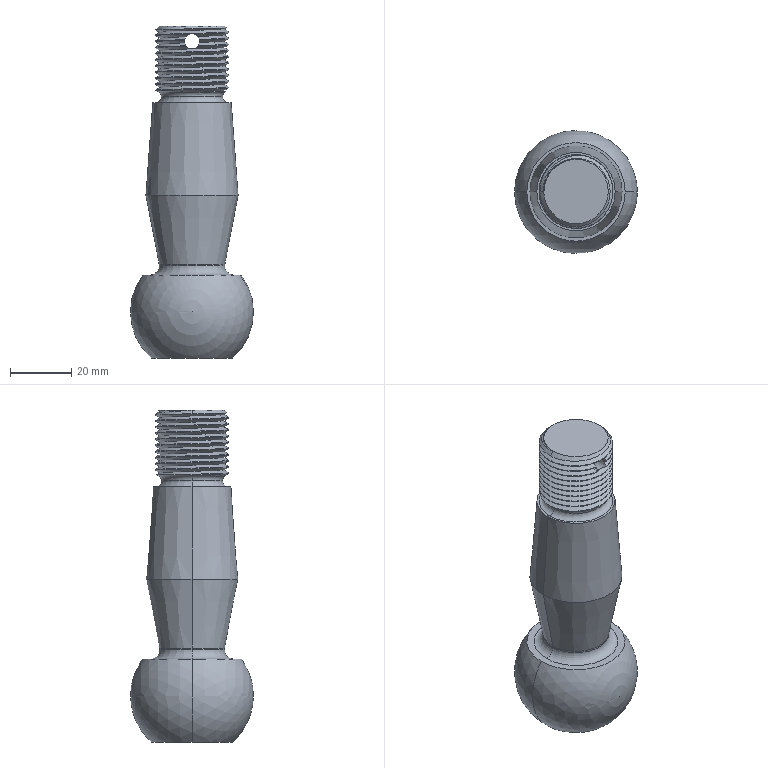Part | SolidWorks | features Chamfer 1, Helix 1, ICE 1, Revolution 1, SweepCut 1 | 1 solid | 60 faces | box 40 x 40 x 108 mm | volume 69235 mm3 | cylinder 26 | spline 12 | torus 8 | cone 7 | plane 5 | sphere 2 | commonest cylinder face diameters 24 x24 5 x2